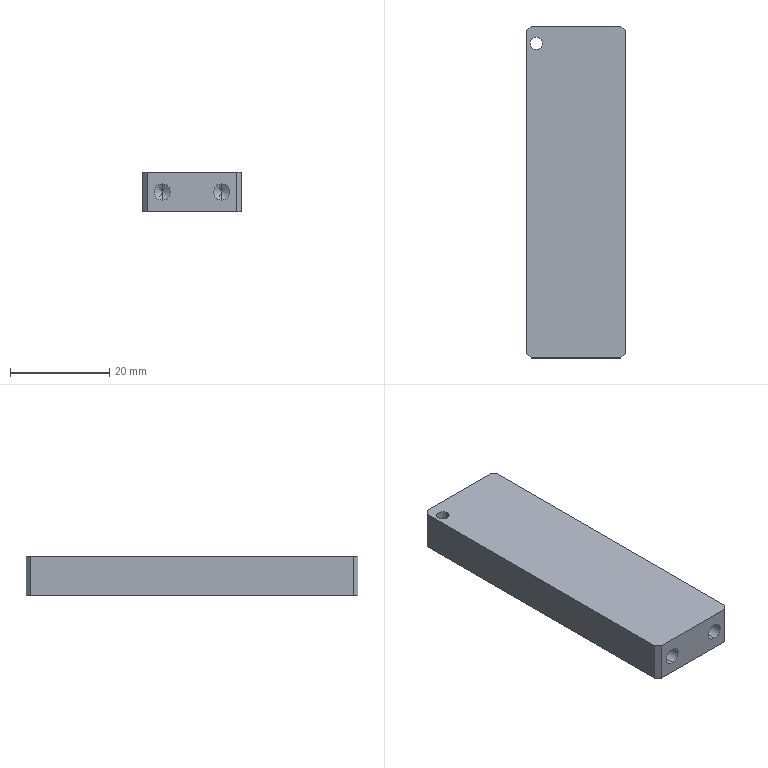Part | SolidWorks | features HoleWzd 2, Chamfer 1, Extrusion 1 | 1 solid | 20 faces | box 20 x 67 x 8 mm | volume 10486 mm3 | plane 10 | cylinder 6 | cone 4 | commonest cylinder face diameters 3.3 x4 2.5 x2
STEP:
#1=CARTESIAN_POINT('',(-6.,-23.4,1.65));
#2=VERTEX_POINT('',#1);
#3=CARTESIAN_POINT('',(-6.,-23.4,-1.65));
#4=VERTEX_POINT('',#3);
#5=CARTESIAN_POINT('',(-6.,-23.4,0.));
#6=DIRECTION('',(0.,-1.,0.));
#7=DIRECTION('',(0.,0.,-1.));
#8=AXIS2_PLACEMENT_3D('',#5,#6,#7);
#9=CIRCLE('',#8,1.65);
#10=EDGE_CURVE('',#2,#4,#9,.T.);
#11=ORIENTED_EDGE('',*,*,#10,.F.);
#12=CARTESIAN_POINT('',(-6.,-33.5,1.65));
#13=VERTEX_POINT('',#12);
#14=CARTESIAN_POINT('',(-6.,-33.5,1.65));
#15=DIRECTION('',(0.,-1.,0.));
#16=VECTOR('',#15,1000.);
#17=LINE('',#14,#16);
#18=EDGE_CURVE('',#2,#13,#17,.T.);
#19=ORIENTED_EDGE('',*,*,#18,.T.);
#20=CARTESIAN_POINT('',(-6.,-33.5,-1.65));
#21=VERTEX_POINT('',#20);
#22=CARTESIAN_POINT('',(-6.,-33.5,0.));
#23=DIRECTION('',(0.,-1.,0.));
#24=DIRECTION('',(0.,0.,-1.));
#25=AXIS2_PLACEMENT_3D('',#22,#23,#24);
#26=CIRCLE('',#25,1.65);
#27=EDGE_CURVE('',#13,#21,#26,.T.);
#28=ORIENTED_EDGE('',*,*,#27,.T.);
#29=CARTESIAN_POINT('',(-6.,-33.5,-1.65));
#30=DIRECTION('',(0.,-1.,0.));
#31=VECTOR('',#30,1000.);
#32=LINE('',#29,#31);
#33=EDGE_CURVE('',#4,#21,#32,.T.);
#34=ORIENTED_EDGE('',*,*,#33,.F.);
#35=EDGE_LOOP('',(#11,#19,#28,#34));
#36=FACE_OUTER_BOUND('',#35,.T.);
#37=CARTESIAN_POINT('',(-6.,-33.5,0.));
#38=DIRECTION('',(0.,-1.,0.));
#39=DIRECTION('',(0.,0.,-1.));
#40=AXIS2_PLACEMENT_3D('',#37,#38,#39);
#41=CYLINDRICAL_SURFACE('',#40,1.65);
#42=ADVANCED_FACE('',(#36),#41,.F.);
#43=CARTESIAN_POINT('',(-6.,-22.409,0.));
#44=VERTEX_POINT('',#43);
#45=CARTESIAN_POINT('',(-6.,-23.4,-1.65));
#46=DIRECTION('',(0.,-0.515,-0.8572));
#47=VECTOR('',#46,1000.);
#48=LINE('',#45,#47);
#49=EDGE_CURVE('',#44,#4,#48,.T.);
#50=ORIENTED_EDGE('',*,*,#49,.F.);
#51=CARTESIAN_POINT('',(-6.,-23.4,1.65));
#52=DIRECTION('',(0.,-0.515,0.8572));
#53=VECTOR('',#52,1000.);
#54=LINE('',#51,#53);
#55=EDGE_CURVE('',#44,#2,#54,.T.);
#56=ORIENTED_EDGE('',*,*,#55,.T.);
#57=ORIENTED_EDGE('',*,*,#10,.T.);
#58=EDGE_LOOP('',(#50,#56,#57));
#59=FACE_OUTER_BOUND('',#58,.T.);
#60=CARTESIAN_POINT('',(-6.,-23.4,0.));
#61=DIRECTION('',(0.,-1.,0.));
#62=DIRECTION('',(0.,0.,-1.));
#63=AXIS2_PLACEMENT_3D('',#60,#61,#62);
#64=CONICAL_SURFACE('',#63,1.65,1.03);
#65=ADVANCED_FACE('',(#59),#64,.F.);
#66=CARTESIAN_POINT('',(6.,-23.4,1.65));
#67=VERTEX_POINT('',#66);
#68=CARTESIAN_POINT('',(6.,-23.4,-1.65));
#69=VERTEX_POINT('',#68);
#70=CARTESIAN_POINT('',(6.,-23.4,0.));
#71=DIRECTION('',(0.,-1.,0.));
#72=DIRECTION('',(0.,0.,-1.));
#73=AXIS2_PLACEMENT_3D('',#70,#71,#72);
#74=CIRCLE('',#73,1.65);
#75=EDGE_CURVE('',#67,#69,#74,.T.);
#76=ORIENTED_EDGE('',*,*,#75,.F.);
#77=CARTESIAN_POINT('',(6.,-33.5,1.65));
#78=VERTEX_POINT('',#77);
#79=CARTESIAN_POINT('',(6.,-33.5,1.65));
#80=DIRECTION('',(0.,-1.,0.));
#81=VECTOR('',#80,1000.);
#82=LINE('',#79,#81);
#83=EDGE_CURVE('',#67,#78,#82,.T.);
#84=ORIENTED_EDGE('',*,*,#83,.T.);
#85=CARTESIAN_POINT('',(6.,-33.5,-1.65));
#86=VERTEX_POINT('',#85);
#87=CARTESIAN_POINT('',(6.,-33.5,0.));
#88=DIRECTION('',(0.,-1.,0.));
#89=DIRECTION('',(0.,0.,-1.));
#90=AXIS2_PLACEMENT_3D('',#87,#88,#89);
#91=CIRCLE('',#90,1.65);
#92=EDGE_CURVE('',#78,#86,#91,.T.);
#93=ORIENTED_EDGE('',*,*,#92,.T.);
#94=CARTESIAN_POINT('',(6.,-33.5,-1.65));
#95=DIRECTION('',(0.,-1.,0.));
#96=VECTOR('',#95,1000.);
#97=LINE('',#94,#96);
#98=EDGE_CURVE('',#69,#86,#97,.T.);
#99=ORIENTED_EDGE('',*,*,#98,.F.);
#100=EDGE_LOOP('',(#76,#84,#93,#99));
#101=FACE_OUTER_BOUND('',#100,.T.);
#102=CARTESIAN_POINT('',(6.,-33.5,0.));
#103=DIRECTION('',(0.,-1.,0.));
#104=DIRECTION('',(0.,0.,-1.));
#105=AXIS2_PLACEMENT_3D('',#102,#103,#104);
#106=CYLINDRICAL_SURFACE('',#105,1.65);
#107=ADVANCED_FACE('',(#101),#106,.F.);
#108=CARTESIAN_POINT('',(6.,-22.409,0.));
#109=VERTEX_POINT('',#108);
#110=CARTESIAN_POINT('',(6.,-23.4,-1.65));
#111=DIRECTION('',(0.,-0.515,-0.8572));
#112=VECTOR('',#111,1000.);
#113=LINE('',#110,#112);
#114=EDGE_CURVE('',#109,#69,#113,.T.);
#115=ORIENTED_EDGE('',*,*,#114,.F.);
#116=CARTESIAN_POINT('',(6.,-23.4,1.65));
#117=DIRECTION('',(0.,-0.515,0.8572));
#118=VECTOR('',#117,1000.);
#119=LINE('',#116,#118);
#120=EDGE_CURVE('',#109,#67,#119,.T.);
#121=ORIENTED_EDGE('',*,*,#120,.T.);
#122=ORIENTED_EDGE('',*,*,#75,.T.);
#123=EDGE_LOOP('',(#115,#121,#122));
#124=FACE_OUTER_BOUND('',#123,.T.);
#125=CARTESIAN_POINT('',(6.,-23.4,0.));
#126=DIRECTION('',(0.,-1.,0.));
#127=DIRECTION('',(0.,0.,-1.));
#128=AXIS2_PLACEMENT_3D('',#125,#126,#127);
#129=CONICAL_SURFACE('',#128,1.65,1.03);
#130=ADVANCED_FACE('',(#124),#129,.F.);
#131=CARTESIAN_POINT('',(-6.75,30.,4.));
#132=VERTEX_POINT('',#131);
#133=CARTESIAN_POINT('',(-9.25,30.,4.));
#134=VERTEX_POINT('',#133);
#135=CARTESIAN_POINT('',(-8.,30.,4.));
#136=DIRECTION('',(0.,0.,-1.));
#137=DIRECTION('',(-1.,0.,0.));
#138=AXIS2_PLACEMENT_3D('',#135,#136,#137);
#139=CIRCLE('',#138,1.25);
#140=EDGE_CURVE('',#132,#134,#139,.T.);
#141=ORIENTED_EDGE('',*,*,#140,.F.);
#142=CARTESIAN_POINT('',(-6.75,30.,-4.));
#143=VERTEX_POINT('',#142);
#144=CARTESIAN_POINT('',(-6.75,30.,-4.));
#145=DIRECTION('',(0.,0.,-1.));
#146=VECTOR('',#145,1000.);
#147=LINE('',#144,#146);
#148=EDGE_CURVE('',#132,#143,#147,.T.);
#149=ORIENTED_EDGE('',*,*,#148,.T.);
#150=CARTESIAN_POINT('',(-9.25,30.,-4.));
#151=VERTEX_POINT('',#150);
#152=CARTESIAN_POINT('',(-8.,30.,-4.));
#153=DIRECTION('',(0.,0.,-1.));
#154=DIRECTION('',(-1.,0.,0.));
#155=AXIS2_PLACEMENT_3D('',#152,#153,#154);
#156=CIRCLE('',#155,1.25);
#157=EDGE_CURVE('',#143,#151,#156,.T.);
#158=ORIENTED_EDGE('',*,*,#157,.T.);
#159=CARTESIAN_POINT('',(-9.25,30.,-4.));
#160=DIRECTION('',(0.,0.,-1.));
#161=VECTOR('',#160,1000.);
#162=LINE('',#159,#161);
#163=EDGE_CURVE('',#134,#151,#162,.T.);
#164=ORIENTED_EDGE('',*,*,#163,.F.);
#165=EDGE_LOOP('',(#141,#149,#158,#164));
#166=FACE_OUTER_BOUND('',#165,.T.);
#167=CARTESIAN_POINT('',(-8.,30.,-4.));
#168=DIRECTION('',(0.,0.,-1.));
#169=DIRECTION('',(-1.,0.,0.));
#170=AXIS2_PLACEMENT_3D('',#167,#168,#169);
#171=CYLINDRICAL_SURFACE('',#170,1.25);
#172=ADVANCED_FACE('',(#166),#171,.F.);
#173=CARTESIAN_POINT('',(10.,-32.5,4.));
#174=VERTEX_POINT('',#173);
#175=CARTESIAN_POINT('',(10.,32.5,4.));
#176=VERTEX_POINT('',#175);
#177=CARTESIAN_POINT('',(10.,33.5,4.));
#178=DIRECTION('',(0.,1.,0.));
#179=VECTOR('',#178,1000.);
#180=LINE('',#177,#179);
#181=EDGE_CURVE('',#174,#176,#180,.T.);
#182=ORIENTED_EDGE('',*,*,#181,.F.);
#183=CARTESIAN_POINT('',(10.,-32.5,-4.));
#184=VERTEX_POINT('',#183);
#185=CARTESIAN_POINT('',(10.,-32.5,4.));
#186=DIRECTION('',(0.,0.,-1.));
#187=VECTOR('',#186,1000.);
#188=LINE('',#185,#187);
#189=EDGE_CURVE('',#174,#184,#188,.T.);
#190=ORIENTED_EDGE('',*,*,#189,.T.);
#191=CARTESIAN_POINT('',(10.,32.5,-4.));
#192=VERTEX_POINT('',#191);
#193=CARTESIAN_POINT('',(10.,33.5,-4.));
#194=DIRECTION('',(0.,1.,0.));
#195=VECTOR('',#194,1000.);
#196=LINE('',#193,#195);
#197=EDGE_CURVE('',#184,#192,#196,.T.);
#198=ORIENTED_EDGE('',*,*,#197,.T.);
#199=CARTESIAN_POINT('',(10.,32.5,4.));
#200=DIRECTION('',(0.,0.,1.));
#201=VECTOR('',#200,1000.);
#202=LINE('',#199,#201);
#203=EDGE_CURVE('',#192,#176,#202,.T.);
#204=ORIENTED_EDGE('',*,*,#203,.T.);
#205=EDGE_LOOP('',(#182,#190,#198,#204));
#206=FACE_OUTER_BOUND('',#205,.T.);
#207=CARTESIAN_POINT('',(10.,33.5,4.));
#208=DIRECTION('',(-1.,0.,0.));
#209=DIRECTION('',(0.,-1.,0.));
#210=AXIS2_PLACEMENT_3D('',#207,#208,#209);
#211=PLANE('',#210);
#212=ADVANCED_FACE('',(#206),#211,.F.);
#213=CARTESIAN_POINT('',(9.,33.5,4.));
#214=VERTEX_POINT('',#213);
#215=CARTESIAN_POINT('',(-9.,33.5,4.));
#216=VERTEX_POINT('',#215);
#217=CARTESIAN_POINT('',(-10.,33.5,4.));
#218=DIRECTION('',(-1.,0.,0.));
#219=VECTOR('',#218,1000.);
#220=LINE('',#217,#219);
#221=EDGE_CURVE('',#214,#216,#220,.T.);
#222=ORIENTED_EDGE('',*,*,#221,.F.);
#223=CARTESIAN_POINT('',(9.,33.5,-4.));
#224=VERTEX_POINT('',#223);
#225=CARTESIAN_POINT('',(9.,33.5,4.));
#226=DIRECTION('',(0.,0.,-1.));
#227=VECTOR('',#226,1000.);
#228=LINE('',#225,#227);
#229=EDGE_CURVE('',#214,#224,#228,.T.);
#230=ORIENTED_EDGE('',*,*,#229,.T.);
#231=CARTESIAN_POINT('',(-9.,33.5,-4.));
#232=VERTEX_POINT('',#231);
#233=CARTESIAN_POINT('',(-10.,33.5,-4.));
#234=DIRECTION('',(-1.,0.,0.));
#235=VECTOR('',#234,1000.);
#236=LINE('',#233,#235);
#237=EDGE_CURVE('',#224,#232,#236,.T.);
#238=ORIENTED_EDGE('',*,*,#237,.T.);
#239=CARTESIAN_POINT('',(-9.,33.5,4.));
#240=DIRECTION('',(0.,0.,1.));
#241=VECTOR('',#240,1000.);
#242=LINE('',#239,#241);
#243=EDGE_CURVE('',#232,#216,#242,.T.);
#244=ORIENTED_EDGE('',*,*,#243,.T.);
#245=EDGE_LOOP('',(#222,#230,#238,#244));
#246=FACE_OUTER_BOUND('',#245,.T.);
#247=CARTESIAN_POINT('',(-10.,33.5,4.));
#248=DIRECTION('',(0.,-1.,0.));
#249=DIRECTION('',(0.,0.,-1.));
#250=AXIS2_PLACEMENT_3D('',#247,#248,#249);
#251=PLANE('',#250);
#252=ADVANCED_FACE('',(#246),#251,.F.);
#253=CARTESIAN_POINT('',(-10.,32.5,-4.));
#254=VERTEX_POINT('',#253);
#255=CARTESIAN_POINT('',(-10.,-32.5,-4.));
#256=VERTEX_POINT('',#255);
#257=CARTESIAN_POINT('',(-10.,33.5,-4.));
#258=DIRECTION('',(0.,-1.,0.));
#259=VECTOR('',#258,1000.);
#260=LINE('',#257,#259);
#261=EDGE_CURVE('',#254,#256,#260,.T.);
#262=ORIENTED_EDGE('',*,*,#261,.T.);
#263=CARTESIAN_POINT('',(-10.,-32.5,4.));
#264=VERTEX_POINT('',#263);
#265=CARTESIAN_POINT('',(-10.,-32.5,4.));
#266=DIRECTION('',(0.,0.,1.));
#267=VECTOR('',#266,1000.);
#268=LINE('',#265,#267);
#269=EDGE_CURVE('',#256,#264,#268,.T.);
#270=ORIENTED_EDGE('',*,*,#269,.T.);
#271=CARTESIAN_POINT('',(-10.,32.5,4.));
#272=VERTEX_POINT('',#271);
#273=CARTESIAN_POINT('',(-10.,33.5,4.));
#274=DIRECTION('',(0.,-1.,0.));
#275=VECTOR('',#274,1000.);
#276=LINE('',#273,#275);
#277=EDGE_CURVE('',#272,#264,#276,.T.);
#278=ORIENTED_EDGE('',*,*,#277,.F.);
#279=CARTESIAN_POINT('',(-10.,32.5,4.));
#280=DIRECTION('',(0.,0.,-1.));
#281=VECTOR('',#280,1000.);
#282=LINE('',#279,#281);
#283=EDGE_CURVE('',#272,#254,#282,.T.);
#284=ORIENTED_EDGE('',*,*,#283,.T.);
#285=EDGE_LOOP('',(#262,#270,#278,#284));
#286=FACE_OUTER_BOUND('',#285,.T.);
#287=CARTESIAN_POINT('',(-10.,33.5,4.));
#288=DIRECTION('',(1.,0.,0.));
#289=DIRECTION('',(0.,1.,0.));
#290=AXIS2_PLACEMENT_3D('',#287,#288,#289);
#291=PLANE('',#290);
#292=ADVANCED_FACE('',(#286),#291,.F.);
#293=CARTESIAN_POINT('',(-6.,-33.5,0.));
#294=DIRECTION('',(0.,-1.,0.));
#295=DIRECTION('',(0.,0.,-1.));
#296=AXIS2_PLACEMENT_3D('',#293,#294,#295);
#297=CIRCLE('',#296,1.65);
#298=EDGE_CURVE('',#21,#13,#297,.T.);
#299=ORIENTED_EDGE('',*,*,#298,.F.);
#300=ORIENTED_EDGE('',*,*,#27,.F.);
#301=EDGE_LOOP('',(#299,#300));
#302=FACE_BOUND('',#301,.T.);
#303=CARTESIAN_POINT('',(6.,-33.5,0.));
#304=DIRECTION('',(0.,-1.,0.));
#305=DIRECTION('',(0.,0.,-1.));
#306=AXIS2_PLACEMENT_3D('',#303,#304,#305);
#307=CIRCLE('',#306,1.65);
#308=EDGE_CURVE('',#86,#78,#307,.T.);
#309=ORIENTED_EDGE('',*,*,#308,.F.);
#310=ORIENTED_EDGE('',*,*,#92,.F.);
#311=EDGE_LOOP('',(#309,#310));
#312=FACE_BOUND('',#311,.T.);
#313=CARTESIAN_POINT('',(-9.,-33.5,4.));
#314=VERTEX_POINT('',#313);
#315=CARTESIAN_POINT('',(9.,-33.5,4.));
#316=VERTEX_POINT('',#315);
#317=CARTESIAN_POINT('',(-10.,-33.5,4.));
#318=DIRECTION('',(1.,0.,0.));
#319=VECTOR('',#318,1000.);
#320=LINE('',#317,#319);
#321=EDGE_CURVE('',#314,#316,#320,.T.);
#322=ORIENTED_EDGE('',*,*,#321,.F.);
#323=CARTESIAN_POINT('',(-9.,-33.5,-4.));
#324=VERTEX_POINT('',#323);
#325=CARTESIAN_POINT('',(-9.,-33.5,4.));
#326=DIRECTION('',(0.,0.,-1.));
#327=VECTOR('',#326,1000.);
#328=LINE('',#325,#327);
#329=EDGE_CURVE('',#314,#324,#328,.T.);
#330=ORIENTED_EDGE('',*,*,#329,.T.);
#331=CARTESIAN_POINT('',(9.,-33.5,-4.));
#332=VERTEX_POINT('',#331);
#333=CARTESIAN_POINT('',(-10.,-33.5,-4.));
#334=DIRECTION('',(1.,0.,0.));
#335=VECTOR('',#334,1000.);
#336=LINE('',#333,#335);
#337=EDGE_CURVE('',#324,#332,#336,.T.);
#338=ORIENTED_EDGE('',*,*,#337,.T.);
#339=CARTESIAN_POINT('',(9.,-33.5,4.));
#340=DIRECTION('',(0.,0.,1.));
#341=VECTOR('',#340,1000.);
#342=LINE('',#339,#341);
#343=EDGE_CURVE('',#332,#316,#342,.T.);
#344=ORIENTED_EDGE('',*,*,#343,.T.);
#345=EDGE_LOOP('',(#322,#330,#338,#344));
#346=FACE_OUTER_BOUND('',#345,.T.);
#347=CARTESIAN_POINT('',(-10.,-33.5,4.));
#348=DIRECTION('',(0.,1.,0.));
#349=DIRECTION('',(0.,0.,1.));
#350=AXIS2_PLACEMENT_3D('',#347,#348,#349);
#351=PLANE('',#350);
#352=ADVANCED_FACE('',(#302,#312,#346),#351,.F.);
#353=CARTESIAN_POINT('',(-8.,30.,4.));
#354=DIRECTION('',(0.,0.,-1.));
#355=DIRECTION('',(-1.,0.,0.));
#356=AXIS2_PLACEMENT_3D('',#353,#354,#355);
#357=CIRCLE('',#356,1.25);
#358=EDGE_CURVE('',#134,#132,#357,.T.);
#359=ORIENTED_EDGE('',*,*,#358,.T.);
#360=ORIENTED_EDGE('',*,*,#140,.T.);
#361=EDGE_LOOP('',(#359,#360));
#362=FACE_BOUND('',#361,.T.);
#363=ORIENTED_EDGE('',*,*,#277,.T.);
#364=CARTESIAN_POINT('',(-21.25,-21.25,4.));
#365=DIRECTION('',(0.7071,-0.7071,0.));
#366=VECTOR('',#365,1000.);
#367=LINE('',#364,#366);
#368=EDGE_CURVE('',#264,#314,#367,.T.);
#369=ORIENTED_EDGE('',*,*,#368,.T.);
#370=ORIENTED_EDGE('',*,*,#321,.T.);
#371=CARTESIAN_POINT('',(21.25,-21.25,4.));
#372=DIRECTION('',(0.7071,0.7071,0.));
#373=VECTOR('',#372,1000.);
#374=LINE('',#371,#373);
#375=EDGE_CURVE('',#316,#174,#374,.T.);
#376=ORIENTED_EDGE('',*,*,#375,.T.);
#377=ORIENTED_EDGE('',*,*,#181,.T.);
#378=CARTESIAN_POINT('',(21.25,21.25,4.));
#379=DIRECTION('',(-0.7071,0.7071,0.));
#380=VECTOR('',#379,1000.);
#381=LINE('',#378,#380);
#382=EDGE_CURVE('',#176,#214,#381,.T.);
#383=ORIENTED_EDGE('',*,*,#382,.T.);
#384=ORIENTED_EDGE('',*,*,#221,.T.);
#385=CARTESIAN_POINT('',(-21.25,21.25,4.));
#386=DIRECTION('',(-0.7071,-0.7071,0.));
#387=VECTOR('',#386,1000.);
#388=LINE('',#385,#387);
#389=EDGE_CURVE('',#216,#272,#388,.T.);
#390=ORIENTED_EDGE('',*,*,#389,.T.);
#391=EDGE_LOOP('',(#363,#369,#370,#376,#377,#383,#384,#390));
#392=FACE_OUTER_BOUND('',#391,.T.);
#393=CARTESIAN_POINT('',(0.,0.,4.));
#394=DIRECTION('',(0.,0.,1.));
#395=DIRECTION('',(1.,0.,0.));
#396=AXIS2_PLACEMENT_3D('',#393,#394,#395);
#397=PLANE('',#396);
#398=ADVANCED_FACE('',(#362,#392),#397,.T.);
#399=CARTESIAN_POINT('',(-8.,30.,-4.));
#400=DIRECTION('',(0.,0.,-1.));
#401=DIRECTION('',(-1.,0.,0.));
#402=AXIS2_PLACEMENT_3D('',#399,#400,#401);
#403=CIRCLE('',#402,1.25);
#404=EDGE_CURVE('',#151,#143,#403,.T.);
#405=ORIENTED_EDGE('',*,*,#404,.F.);
#406=ORIENTED_EDGE('',*,*,#157,.F.);
#407=EDGE_LOOP('',(#405,#406));
#408=FACE_BOUND('',#407,.T.);
#409=ORIENTED_EDGE('',*,*,#337,.F.);
#410=CARTESIAN_POINT('',(-9.,-33.5,-4.));
#411=DIRECTION('',(-0.7071,0.7071,0.));
#412=VECTOR('',#411,1000.);
#413=LINE('',#410,#412);
#414=EDGE_CURVE('',#324,#256,#413,.T.);
#415=ORIENTED_EDGE('',*,*,#414,.T.);
#416=ORIENTED_EDGE('',*,*,#261,.F.);
#417=CARTESIAN_POINT('',(-10.,32.5,-4.));
#418=DIRECTION('',(0.7071,0.7071,0.));
#419=VECTOR('',#418,1000.);
#420=LINE('',#417,#419);
#421=EDGE_CURVE('',#254,#232,#420,.T.);
#422=ORIENTED_EDGE('',*,*,#421,.T.);
#423=ORIENTED_EDGE('',*,*,#237,.F.);
#424=CARTESIAN_POINT('',(9.,33.5,-4.));
#425=DIRECTION('',(0.7071,-0.7071,0.));
#426=VECTOR('',#425,1000.);
#427=LINE('',#424,#426);
#428=EDGE_CURVE('',#224,#192,#427,.T.);
#429=ORIENTED_EDGE('',*,*,#428,.T.);
#430=ORIENTED_EDGE('',*,*,#197,.F.);
#431=CARTESIAN_POINT('',(10.,-32.5,-4.));
#432=DIRECTION('',(-0.7071,-0.7071,0.));
#433=VECTOR('',#432,1000.);
#434=LINE('',#431,#433);
#435=EDGE_CURVE('',#184,#332,#434,.T.);
#436=ORIENTED_EDGE('',*,*,#435,.T.);
#437=EDGE_LOOP('',(#409,#415,#416,#422,#423,#429,#430,#436));
#438=FACE_OUTER_BOUND('',#437,.T.);
#439=CARTESIAN_POINT('',(0.,0.,-4.));
#440=DIRECTION('',(0.,0.,1.));
#441=DIRECTION('',(1.,0.,0.));
#442=AXIS2_PLACEMENT_3D('',#439,#440,#441);
#443=PLANE('',#442);
#444=ADVANCED_FACE('',(#408,#438),#443,.F.);
#445=ORIENTED_EDGE('',*,*,#148,.F.);
#446=ORIENTED_EDGE('',*,*,#358,.F.);
#447=ORIENTED_EDGE('',*,*,#163,.T.);
#448=ORIENTED_EDGE('',*,*,#404,.T.);
#449=EDGE_LOOP('',(#445,#446,#447,#448));
#450=FACE_OUTER_BOUND('',#449,.T.);
#451=CARTESIAN_POINT('',(-8.,30.,-4.));
#452=DIRECTION('',(0.,0.,-1.));
#453=DIRECTION('',(-1.,0.,0.));
#454=AXIS2_PLACEMENT_3D('',#451,#452,#453);
#455=CYLINDRICAL_SURFACE('',#454,1.25);
#456=ADVANCED_FACE('',(#450),#455,.F.);
#457=ORIENTED_EDGE('',*,*,#120,.F.);
#458=ORIENTED_EDGE('',*,*,#114,.T.);
#459=CARTESIAN_POINT('',(6.,-23.4,0.));
#460=DIRECTION('',(0.,-1.,0.));
#461=DIRECTION('',(0.,0.,-1.));
#462=AXIS2_PLACEMENT_3D('',#459,#460,#461);
#463=CIRCLE('',#462,1.65);
#464=EDGE_CURVE('',#69,#67,#463,.T.);
#465=ORIENTED_EDGE('',*,*,#464,.T.);
#466=EDGE_LOOP('',(#457,#458,#465));
#467=FACE_OUTER_BOUND('',#466,.T.);
#468=CARTESIAN_POINT('',(6.,-23.4,0.));
#469=DIRECTION('',(0.,-1.,0.));
#470=DIRECTION('',(0.,0.,-1.));
#471=AXIS2_PLACEMENT_3D('',#468,#469,#470);
#472=CONICAL_SURFACE('',#471,1.65,1.03);
#473=ADVANCED_FACE('',(#467),#472,.F.);
#474=ORIENTED_EDGE('',*,*,#83,.F.);
#475=ORIENTED_EDGE('',*,*,#464,.F.);
#476=ORIENTED_EDGE('',*,*,#98,.T.);
#477=ORIENTED_EDGE('',*,*,#308,.T.);
#478=EDGE_LOOP('',(#474,#475,#476,#477));
#479=FACE_OUTER_BOUND('',#478,.T.);
#480=CARTESIAN_POINT('',(6.,-33.5,0.));
#481=DIRECTION('',(0.,-1.,0.));
#482=DIRECTION('',(0.,0.,-1.));
#483=AXIS2_PLACEMENT_3D('',#480,#481,#482);
#484=CYLINDRICAL_SURFACE('',#483,1.65);
#485=ADVANCED_FACE('',(#479),#484,.F.);
#486=ORIENTED_EDGE('',*,*,#55,.F.);
#487=ORIENTED_EDGE('',*,*,#49,.T.);
#488=CARTESIAN_POINT('',(-6.,-23.4,0.));
#489=DIRECTION('',(0.,-1.,0.));
#490=DIRECTION('',(0.,0.,-1.));
#491=AXIS2_PLACEMENT_3D('',#488,#489,#490);
#492=CIRCLE('',#491,1.65);
#493=EDGE_CURVE('',#4,#2,#492,.T.);
#494=ORIENTED_EDGE('',*,*,#493,.T.);
#495=EDGE_LOOP('',(#486,#487,#494));
#496=FACE_OUTER_BOUND('',#495,.T.);
#497=CARTESIAN_POINT('',(-6.,-23.4,0.));
#498=DIRECTION('',(0.,-1.,0.));
#499=DIRECTION('',(0.,0.,-1.));
#500=AXIS2_PLACEMENT_3D('',#497,#498,#499);
#501=CONICAL_SURFACE('',#500,1.65,1.03);
#502=ADVANCED_FACE('',(#496),#501,.F.);
#503=ORIENTED_EDGE('',*,*,#18,.F.);
#504=ORIENTED_EDGE('',*,*,#493,.F.);
#505=ORIENTED_EDGE('',*,*,#33,.T.);
#506=ORIENTED_EDGE('',*,*,#298,.T.);
#507=EDGE_LOOP('',(#503,#504,#505,#506));
#508=FACE_OUTER_BOUND('',#507,.T.);
#509=CARTESIAN_POINT('',(-6.,-33.5,0.));
#510=DIRECTION('',(0.,-1.,0.));
#511=DIRECTION('',(0.,0.,-1.));
#512=AXIS2_PLACEMENT_3D('',#509,#510,#511);
#513=CYLINDRICAL_SURFACE('',#512,1.65);
#514=ADVANCED_FACE('',(#508),#513,.F.);
#515=ORIENTED_EDGE('',*,*,#368,.F.);
#516=ORIENTED_EDGE('',*,*,#269,.F.);
#517=ORIENTED_EDGE('',*,*,#414,.F.);
#518=ORIENTED_EDGE('',*,*,#329,.F.);
#519=EDGE_LOOP('',(#515,#516,#517,#518));
#520=FACE_OUTER_BOUND('',#519,.T.);
#521=CARTESIAN_POINT('',(-9.,-33.5,4.));
#522=DIRECTION('',(0.7071,0.7071,0.));
#523=DIRECTION('',(0.,0.,-1.));
#524=AXIS2_PLACEMENT_3D('',#521,#522,#523);
#525=PLANE('',#524);
#526=ADVANCED_FACE('',(#520),#525,.F.);
#527=ORIENTED_EDGE('',*,*,#375,.F.);
#528=ORIENTED_EDGE('',*,*,#343,.F.);
#529=ORIENTED_EDGE('',*,*,#435,.F.);
#530=ORIENTED_EDGE('',*,*,#189,.F.);
#531=EDGE_LOOP('',(#527,#528,#529,#530));
#532=FACE_OUTER_BOUND('',#531,.T.);
#533=CARTESIAN_POINT('',(10.,-32.5,4.));
#534=DIRECTION('',(-0.7071,0.7071,0.));
#535=DIRECTION('',(0.,0.,-1.));
#536=AXIS2_PLACEMENT_3D('',#533,#534,#535);
#537=PLANE('',#536);
#538=ADVANCED_FACE('',(#532),#537,.F.);
#539=ORIENTED_EDGE('',*,*,#382,.F.);
#540=ORIENTED_EDGE('',*,*,#203,.F.);
#541=ORIENTED_EDGE('',*,*,#428,.F.);
#542=ORIENTED_EDGE('',*,*,#229,.F.);
#543=EDGE_LOOP('',(#539,#540,#541,#542));
#544=FACE_OUTER_BOUND('',#543,.T.);
#545=CARTESIAN_POINT('',(9.,33.5,4.));
#546=DIRECTION('',(-0.7071,-0.7071,0.));
#547=DIRECTION('',(0.,0.,-1.));
#548=AXIS2_PLACEMENT_3D('',#545,#546,#547);
#549=PLANE('',#548);
#550=ADVANCED_FACE('',(#544),#549,.F.);
#551=ORIENTED_EDGE('',*,*,#389,.F.);
#552=ORIENTED_EDGE('',*,*,#243,.F.);
#553=ORIENTED_EDGE('',*,*,#421,.F.);
#554=ORIENTED_EDGE('',*,*,#283,.F.);
#555=EDGE_LOOP('',(#551,#552,#553,#554));
#556=FACE_OUTER_BOUND('',#555,.T.);
#557=CARTESIAN_POINT('',(-10.,32.5,4.));
#558=DIRECTION('',(0.7071,-0.7071,0.));
#559=DIRECTION('',(0.,0.,-1.));
#560=AXIS2_PLACEMENT_3D('',#557,#558,#559);
#561=PLANE('',#560);
#562=ADVANCED_FACE('',(#556),#561,.F.);
#563=CLOSED_SHELL('',(#42,#65,#107,#130,#172,#212,#252,#292,#352,#398,#444,#456,#473,#485,#502,#514,#526,#538,#550,#562));
#564=MANIFOLD_SOLID_BREP('',#563);
#565=CARTESIAN_POINT('',(0.,0.,0.));
#566=DIRECTION('',(0.,0.,1.));
#567=DIRECTION('',(1.,0.,0.));
#568=AXIS2_PLACEMENT_3D('',#565,#566,#567);
#569=(LENGTH_UNIT()NAMED_UNIT(*)SI_UNIT(.MILLI.,.METRE.));
#570=UNCERTAINTY_MEASURE_WITH_UNIT(LENGTH_MEASURE(0.00001),#569,'','');
#571=(NAMED_UNIT(*)PLANE_ANGLE_UNIT()SI_UNIT($,.RADIAN.));
#572=(NAMED_UNIT(*)SI_UNIT($,.STERADIAN.)SOLID_ANGLE_UNIT());
#573=(GEOMETRIC_REPRESENTATION_CONTEXT(3)GLOBAL_UNCERTAINTY_ASSIGNED_CONTEXT((#570))GLOBAL_UNIT_ASSIGNED_CONTEXT((#569,#571,#572))REPRESENTATION_CONTEXT('',''));
#574=ADVANCED_BREP_SHAPE_REPRESENTATION('',(#564,#568),#573);